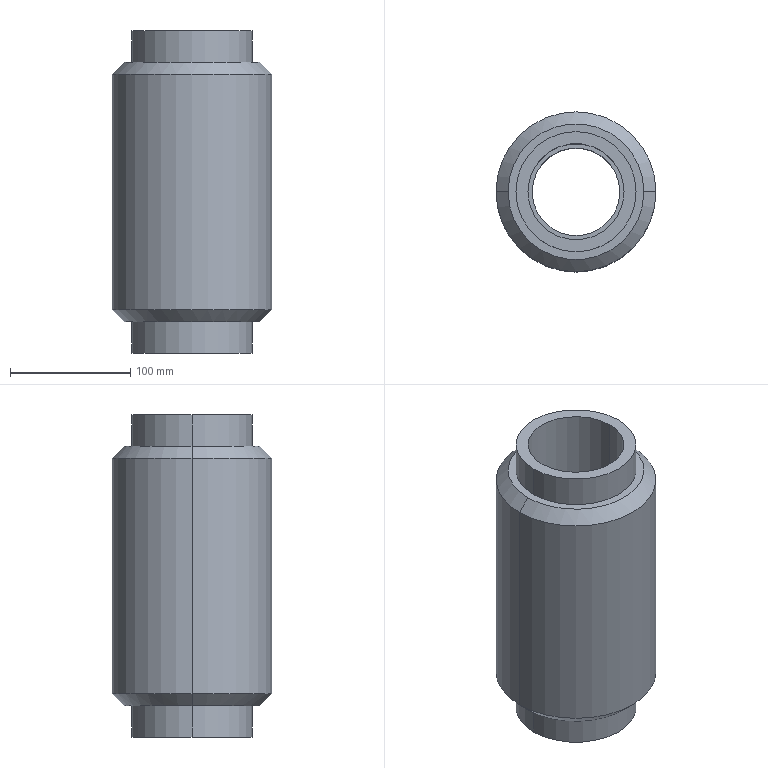Part | SolidWorks | features ICE 5, Chamfer 2, Extrusion 1 | 1 solid | 22 faces | box 133 x 133 x 268 mm | volume 2114999 mm3 | cylinder 12 | plane 6 | cone 4 | commonest cylinder face diameters 80 x4 100 x4 73 x2 133 x2
STEP:
#1=CARTESIAN_POINT('',(-56.5,0.,26.));
#2=VERTEX_POINT('',#1);
#3=CARTESIAN_POINT('',(56.5,0.,26.));
#4=VERTEX_POINT('',#3);
#5=CARTESIAN_POINT('',(0.,0.,26.));
#6=DIRECTION('',(0.,0.,-1.));
#7=DIRECTION('',(1.,0.,0.));
#8=AXIS2_PLACEMENT_3D('',#5,#6,#7);
#9=CIRCLE('',#8,56.5);
#10=EDGE_CURVE('',#2,#4,#9,.T.);
#11=ORIENTED_EDGE('',*,*,#10,.F.);
#12=CARTESIAN_POINT('',(-66.5,0.,36.));
#13=VERTEX_POINT('',#12);
#14=CARTESIAN_POINT('',(-66.5,0.,36.));
#15=DIRECTION('',(-0.7071,0.,0.7071));
#16=VECTOR('',#15,1000.);
#17=LINE('',#14,#16);
#18=EDGE_CURVE('',#2,#13,#17,.T.);
#19=ORIENTED_EDGE('',*,*,#18,.T.);
#20=CARTESIAN_POINT('',(66.5,0.,36.));
#21=VERTEX_POINT('',#20);
#22=CARTESIAN_POINT('',(0.,0.,36.));
#23=DIRECTION('',(0.,0.,1.));
#24=DIRECTION('',(1.,0.,0.));
#25=AXIS2_PLACEMENT_3D('',#22,#23,#24);
#26=CIRCLE('',#25,66.5);
#27=EDGE_CURVE('',#21,#13,#26,.T.);
#28=ORIENTED_EDGE('',*,*,#27,.F.);
#29=CARTESIAN_POINT('',(66.5,0.,36.));
#30=DIRECTION('',(0.7071,0.,0.7071));
#31=VECTOR('',#30,1000.);
#32=LINE('',#29,#31);
#33=EDGE_CURVE('',#4,#21,#32,.T.);
#34=ORIENTED_EDGE('',*,*,#33,.F.);
#35=EDGE_LOOP('',(#11,#19,#28,#34));
#36=FACE_OUTER_BOUND('',#35,.T.);
#37=CARTESIAN_POINT('',(0.,0.,36.));
#38=DIRECTION('',(0.,0.,1.));
#39=DIRECTION('',(1.,0.,0.));
#40=AXIS2_PLACEMENT_3D('',#37,#38,#39);
#41=CONICAL_SURFACE('',#40,66.5,0.7854);
#42=ADVANCED_FACE('',(#36),#41,.T.);
#43=CARTESIAN_POINT('',(56.5,0.,242.));
#44=VERTEX_POINT('',#43);
#45=CARTESIAN_POINT('',(-56.5,0.,242.));
#46=VERTEX_POINT('',#45);
#47=CARTESIAN_POINT('',(0.,0.,242.));
#48=DIRECTION('',(0.,0.,1.));
#49=DIRECTION('',(1.,0.,0.));
#50=AXIS2_PLACEMENT_3D('',#47,#48,#49);
#51=CIRCLE('',#50,56.5);
#52=EDGE_CURVE('',#44,#46,#51,.T.);
#53=ORIENTED_EDGE('',*,*,#52,.F.);
#54=CARTESIAN_POINT('',(66.5,0.,232.));
#55=VERTEX_POINT('',#54);
#56=CARTESIAN_POINT('',(56.5,0.,242.));
#57=DIRECTION('',(0.7071,0.,-0.7071));
#58=VECTOR('',#57,1000.);
#59=LINE('',#56,#58);
#60=EDGE_CURVE('',#44,#55,#59,.T.);
#61=ORIENTED_EDGE('',*,*,#60,.T.);
#62=CARTESIAN_POINT('',(-66.5,0.,232.));
#63=VERTEX_POINT('',#62);
#64=CARTESIAN_POINT('',(0.,0.,232.));
#65=DIRECTION('',(0.,0.,-1.));
#66=DIRECTION('',(1.,0.,0.));
#67=AXIS2_PLACEMENT_3D('',#64,#65,#66);
#68=CIRCLE('',#67,66.5);
#69=EDGE_CURVE('',#63,#55,#68,.T.);
#70=ORIENTED_EDGE('',*,*,#69,.F.);
#71=CARTESIAN_POINT('',(-56.5,0.,242.));
#72=DIRECTION('',(-0.7071,0.,-0.7071));
#73=VECTOR('',#72,1000.);
#74=LINE('',#71,#73);
#75=EDGE_CURVE('',#46,#63,#74,.T.);
#76=ORIENTED_EDGE('',*,*,#75,.F.);
#77=EDGE_LOOP('',(#53,#61,#70,#76));
#78=FACE_OUTER_BOUND('',#77,.T.);
#79=CARTESIAN_POINT('',(0.,0.,242.));
#80=DIRECTION('',(0.,0.,-1.));
#81=DIRECTION('',(-1.,0.,0.));
#82=AXIS2_PLACEMENT_3D('',#79,#80,#81);
#83=CONICAL_SURFACE('',#82,56.5,0.7854);
#84=ADVANCED_FACE('',(#78),#83,.T.);
#85=CARTESIAN_POINT('',(-36.5,0.,189.));
#86=VERTEX_POINT('',#85);
#87=CARTESIAN_POINT('',(36.5,0.,189.));
#88=VERTEX_POINT('',#87);
#89=CARTESIAN_POINT('',(0.,0.,189.));
#90=DIRECTION('',(0.,0.,1.));
#91=DIRECTION('',(1.,0.,0.));
#92=AXIS2_PLACEMENT_3D('',#89,#90,#91);
#93=CIRCLE('',#92,36.5);
#94=EDGE_CURVE('',#86,#88,#93,.T.);
#95=ORIENTED_EDGE('',*,*,#94,.T.);
#96=CARTESIAN_POINT('',(36.5,0.,79.));
#97=VERTEX_POINT('',#96);
#98=CARTESIAN_POINT('',(36.5,0.,268.));
#99=DIRECTION('',(0.,0.,-1.));
#100=VECTOR('',#99,1000.);
#101=LINE('',#98,#100);
#102=EDGE_CURVE('',#88,#97,#101,.T.);
#103=ORIENTED_EDGE('',*,*,#102,.T.);
#104=CARTESIAN_POINT('',(-36.5,0.,79.));
#105=VERTEX_POINT('',#104);
#106=CARTESIAN_POINT('',(0.,0.,79.));
#107=DIRECTION('',(0.,0.,-1.));
#108=DIRECTION('',(-1.,0.,0.));
#109=AXIS2_PLACEMENT_3D('',#106,#107,#108);
#110=CIRCLE('',#109,36.5);
#111=EDGE_CURVE('',#97,#105,#110,.T.);
#112=ORIENTED_EDGE('',*,*,#111,.T.);
#113=CARTESIAN_POINT('',(-36.5,0.,268.));
#114=DIRECTION('',(0.,0.,-1.));
#115=VECTOR('',#114,1000.);
#116=LINE('',#113,#115);
#117=EDGE_CURVE('',#86,#105,#116,.T.);
#118=ORIENTED_EDGE('',*,*,#117,.F.);
#119=EDGE_LOOP('',(#95,#103,#112,#118));
#120=FACE_OUTER_BOUND('',#119,.T.);
#121=CARTESIAN_POINT('',(0.,0.,268.));
#122=DIRECTION('',(0.,0.,-1.));
#123=DIRECTION('',(-1.,0.,0.));
#124=AXIS2_PLACEMENT_3D('',#121,#122,#123);
#125=CYLINDRICAL_SURFACE('',#124,36.5);
#126=ADVANCED_FACE('',(#120),#125,.F.);
#127=CARTESIAN_POINT('',(40.,0.,79.));
#128=VERTEX_POINT('',#127);
#129=CARTESIAN_POINT('',(-40.,0.,79.));
#130=VERTEX_POINT('',#129);
#131=CARTESIAN_POINT('',(0.,0.,79.));
#132=DIRECTION('',(0.,0.,-1.));
#133=DIRECTION('',(-1.,0.,0.));
#134=AXIS2_PLACEMENT_3D('',#131,#132,#133);
#135=CIRCLE('',#134,40.);
#136=EDGE_CURVE('',#128,#130,#135,.T.);
#137=ORIENTED_EDGE('',*,*,#136,.F.);
#138=CARTESIAN_POINT('',(40.,0.,0.));
#139=VERTEX_POINT('',#138);
#140=CARTESIAN_POINT('',(40.,0.,79.));
#141=DIRECTION('',(0.,0.,-1.));
#142=VECTOR('',#141,1000.);
#143=LINE('',#140,#142);
#144=EDGE_CURVE('',#128,#139,#143,.T.);
#145=ORIENTED_EDGE('',*,*,#144,.T.);
#146=CARTESIAN_POINT('',(-40.,0.,0.));
#147=VERTEX_POINT('',#146);
#148=CARTESIAN_POINT('',(0.,0.,0.));
#149=DIRECTION('',(0.,0.,-1.));
#150=DIRECTION('',(-1.,0.,0.));
#151=AXIS2_PLACEMENT_3D('',#148,#149,#150);
#152=CIRCLE('',#151,40.);
#153=EDGE_CURVE('',#139,#147,#152,.T.);
#154=ORIENTED_EDGE('',*,*,#153,.T.);
#155=CARTESIAN_POINT('',(-40.,0.,79.));
#156=DIRECTION('',(0.,0.,-1.));
#157=VECTOR('',#156,1000.);
#158=LINE('',#155,#157);
#159=EDGE_CURVE('',#130,#147,#158,.T.);
#160=ORIENTED_EDGE('',*,*,#159,.F.);
#161=EDGE_LOOP('',(#137,#145,#154,#160));
#162=FACE_OUTER_BOUND('',#161,.T.);
#163=CARTESIAN_POINT('',(0.,0.,79.));
#164=DIRECTION('',(0.,0.,-1.));
#165=DIRECTION('',(-1.,0.,0.));
#166=AXIS2_PLACEMENT_3D('',#163,#164,#165);
#167=CYLINDRICAL_SURFACE('',#166,40.);
#168=ADVANCED_FACE('',(#162),#167,.F.);
#169=CARTESIAN_POINT('',(-40.,0.,189.));
#170=VERTEX_POINT('',#169);
#171=CARTESIAN_POINT('',(40.,0.,189.));
#172=VERTEX_POINT('',#171);
#173=CARTESIAN_POINT('',(0.,0.,189.));
#174=DIRECTION('',(0.,0.,1.));
#175=DIRECTION('',(1.,0.,0.));
#176=AXIS2_PLACEMENT_3D('',#173,#174,#175);
#177=CIRCLE('',#176,40.);
#178=EDGE_CURVE('',#170,#172,#177,.T.);
#179=ORIENTED_EDGE('',*,*,#178,.F.);
#180=CARTESIAN_POINT('',(-40.,0.,268.));
#181=VERTEX_POINT('',#180);
#182=CARTESIAN_POINT('',(-40.,0.,189.));
#183=DIRECTION('',(0.,0.,1.));
#184=VECTOR('',#183,1000.);
#185=LINE('',#182,#184);
#186=EDGE_CURVE('',#170,#181,#185,.T.);
#187=ORIENTED_EDGE('',*,*,#186,.T.);
#188=CARTESIAN_POINT('',(40.,0.,268.));
#189=VERTEX_POINT('',#188);
#190=CARTESIAN_POINT('',(0.,0.,268.));
#191=DIRECTION('',(0.,0.,1.));
#192=DIRECTION('',(1.,0.,0.));
#193=AXIS2_PLACEMENT_3D('',#190,#191,#192);
#194=CIRCLE('',#193,40.);
#195=EDGE_CURVE('',#181,#189,#194,.T.);
#196=ORIENTED_EDGE('',*,*,#195,.T.);
#197=CARTESIAN_POINT('',(40.,0.,189.));
#198=DIRECTION('',(0.,0.,1.));
#199=VECTOR('',#198,1000.);
#200=LINE('',#197,#199);
#201=EDGE_CURVE('',#172,#189,#200,.T.);
#202=ORIENTED_EDGE('',*,*,#201,.F.);
#203=EDGE_LOOP('',(#179,#187,#196,#202));
#204=FACE_OUTER_BOUND('',#203,.T.);
#205=CARTESIAN_POINT('',(0.,0.,189.));
#206=DIRECTION('',(0.,0.,1.));
#207=DIRECTION('',(1.,0.,0.));
#208=AXIS2_PLACEMENT_3D('',#205,#206,#207);
#209=CYLINDRICAL_SURFACE('',#208,40.);
#210=ADVANCED_FACE('',(#204),#209,.F.);
#211=CARTESIAN_POINT('',(50.,0.,268.));
#212=VERTEX_POINT('',#211);
#213=CARTESIAN_POINT('',(-50.,0.,268.));
#214=VERTEX_POINT('',#213);
#215=CARTESIAN_POINT('',(0.,0.,268.));
#216=DIRECTION('',(0.,0.,1.));
#217=DIRECTION('',(1.,0.,0.));
#218=AXIS2_PLACEMENT_3D('',#215,#216,#217);
#219=CIRCLE('',#218,50.);
#220=EDGE_CURVE('',#212,#214,#219,.T.);
#221=ORIENTED_EDGE('',*,*,#220,.F.);
#222=CARTESIAN_POINT('',(50.,0.,242.));
#223=VERTEX_POINT('',#222);
#224=CARTESIAN_POINT('',(50.,0.,268.));
#225=DIRECTION('',(0.,0.,-1.));
#226=VECTOR('',#225,1000.);
#227=LINE('',#224,#226);
#228=EDGE_CURVE('',#212,#223,#227,.T.);
#229=ORIENTED_EDGE('',*,*,#228,.T.);
#230=CARTESIAN_POINT('',(-50.,0.,242.));
#231=VERTEX_POINT('',#230);
#232=CARTESIAN_POINT('',(0.,0.,242.));
#233=DIRECTION('',(0.,0.,1.));
#234=DIRECTION('',(1.,0.,0.));
#235=AXIS2_PLACEMENT_3D('',#232,#233,#234);
#236=CIRCLE('',#235,50.);
#237=EDGE_CURVE('',#223,#231,#236,.T.);
#238=ORIENTED_EDGE('',*,*,#237,.T.);
#239=CARTESIAN_POINT('',(-50.,0.,268.));
#240=DIRECTION('',(0.,0.,-1.));
#241=VECTOR('',#240,1000.);
#242=LINE('',#239,#241);
#243=EDGE_CURVE('',#214,#231,#242,.T.);
#244=ORIENTED_EDGE('',*,*,#243,.F.);
#245=EDGE_LOOP('',(#221,#229,#238,#244));
#246=FACE_OUTER_BOUND('',#245,.T.);
#247=CARTESIAN_POINT('',(0.,0.,268.));
#248=DIRECTION('',(0.,0.,-1.));
#249=DIRECTION('',(-1.,0.,0.));
#250=AXIS2_PLACEMENT_3D('',#247,#248,#249);
#251=CYLINDRICAL_SURFACE('',#250,50.);
#252=ADVANCED_FACE('',(#246),#251,.T.);
#253=ORIENTED_EDGE('',*,*,#69,.T.);
#254=CARTESIAN_POINT('',(66.5,0.,242.));
#255=DIRECTION('',(0.,0.,-1.));
#256=VECTOR('',#255,1000.);
#257=LINE('',#254,#256);
#258=EDGE_CURVE('',#55,#21,#257,.T.);
#259=ORIENTED_EDGE('',*,*,#258,.T.);
#260=ORIENTED_EDGE('',*,*,#27,.T.);
#261=CARTESIAN_POINT('',(-66.5,0.,242.));
#262=DIRECTION('',(0.,0.,-1.));
#263=VECTOR('',#262,1000.);
#264=LINE('',#261,#263);
#265=EDGE_CURVE('',#63,#13,#264,.T.);
#266=ORIENTED_EDGE('',*,*,#265,.F.);
#267=EDGE_LOOP('',(#253,#259,#260,#266));
#268=FACE_OUTER_BOUND('',#267,.T.);
#269=CARTESIAN_POINT('',(0.,0.,242.));
#270=DIRECTION('',(0.,0.,-1.));
#271=DIRECTION('',(-1.,0.,0.));
#272=AXIS2_PLACEMENT_3D('',#269,#270,#271);
#273=CYLINDRICAL_SURFACE('',#272,66.5);
#274=ADVANCED_FACE('',(#268),#273,.T.);
#275=CARTESIAN_POINT('',(50.,0.,26.));
#276=VERTEX_POINT('',#275);
#277=CARTESIAN_POINT('',(-50.,0.,26.));
#278=VERTEX_POINT('',#277);
#279=CARTESIAN_POINT('',(0.,0.,26.));
#280=DIRECTION('',(0.,0.,1.));
#281=DIRECTION('',(1.,0.,0.));
#282=AXIS2_PLACEMENT_3D('',#279,#280,#281);
#283=CIRCLE('',#282,50.);
#284=EDGE_CURVE('',#276,#278,#283,.T.);
#285=ORIENTED_EDGE('',*,*,#284,.F.);
#286=CARTESIAN_POINT('',(50.,0.,0.));
#287=VERTEX_POINT('',#286);
#288=CARTESIAN_POINT('',(50.,0.,26.));
#289=DIRECTION('',(0.,0.,-1.));
#290=VECTOR('',#289,1000.);
#291=LINE('',#288,#290);
#292=EDGE_CURVE('',#276,#287,#291,.T.);
#293=ORIENTED_EDGE('',*,*,#292,.T.);
#294=CARTESIAN_POINT('',(-50.,0.,0.));
#295=VERTEX_POINT('',#294);
#296=CARTESIAN_POINT('',(0.,0.,0.));
#297=DIRECTION('',(0.,0.,1.));
#298=DIRECTION('',(1.,0.,0.));
#299=AXIS2_PLACEMENT_3D('',#296,#297,#298);
#300=CIRCLE('',#299,50.);
#301=EDGE_CURVE('',#287,#295,#300,.T.);
#302=ORIENTED_EDGE('',*,*,#301,.T.);
#303=CARTESIAN_POINT('',(-50.,0.,26.));
#304=DIRECTION('',(0.,0.,-1.));
#305=VECTOR('',#304,1000.);
#306=LINE('',#303,#305);
#307=EDGE_CURVE('',#278,#295,#306,.T.);
#308=ORIENTED_EDGE('',*,*,#307,.F.);
#309=EDGE_LOOP('',(#285,#293,#302,#308));
#310=FACE_OUTER_BOUND('',#309,.T.);
#311=CARTESIAN_POINT('',(0.,0.,26.));
#312=DIRECTION('',(0.,0.,-1.));
#313=DIRECTION('',(-1.,0.,0.));
#314=AXIS2_PLACEMENT_3D('',#311,#312,#313);
#315=CYLINDRICAL_SURFACE('',#314,50.);
#316=ADVANCED_FACE('',(#310),#315,.T.);
#317=CARTESIAN_POINT('',(0.,0.,242.));
#318=DIRECTION('',(0.,0.,1.));
#319=DIRECTION('',(1.,0.,0.));
#320=AXIS2_PLACEMENT_3D('',#317,#318,#319);
#321=CIRCLE('',#320,56.5);
#322=EDGE_CURVE('',#46,#44,#321,.T.);
#323=ORIENTED_EDGE('',*,*,#322,.T.);
#324=ORIENTED_EDGE('',*,*,#52,.T.);
#325=EDGE_LOOP('',(#323,#324));
#326=FACE_OUTER_BOUND('',#325,.T.);
#327=CARTESIAN_POINT('',(0.,0.,242.));
#328=DIRECTION('',(0.,0.,1.));
#329=DIRECTION('',(1.,0.,0.));
#330=AXIS2_PLACEMENT_3D('',#327,#328,#329);
#331=CIRCLE('',#330,50.);
#332=EDGE_CURVE('',#231,#223,#331,.T.);
#333=ORIENTED_EDGE('',*,*,#332,.F.);
#334=ORIENTED_EDGE('',*,*,#237,.F.);
#335=EDGE_LOOP('',(#333,#334));
#336=FACE_BOUND('',#335,.T.);
#337=CARTESIAN_POINT('',(0.,0.,242.));
#338=DIRECTION('',(0.,0.,1.));
#339=DIRECTION('',(1.,0.,0.));
#340=AXIS2_PLACEMENT_3D('',#337,#338,#339);
#341=PLANE('',#340);
#342=ADVANCED_FACE('',(#326,#336),#341,.T.);
#343=ORIENTED_EDGE('',*,*,#292,.F.);
#344=CARTESIAN_POINT('',(0.,0.,26.));
#345=DIRECTION('',(0.,0.,1.));
#346=DIRECTION('',(1.,0.,0.));
#347=AXIS2_PLACEMENT_3D('',#344,#345,#346);
#348=CIRCLE('',#347,50.);
#349=EDGE_CURVE('',#278,#276,#348,.T.);
#350=ORIENTED_EDGE('',*,*,#349,.F.);
#351=ORIENTED_EDGE('',*,*,#307,.T.);
#352=CARTESIAN_POINT('',(0.,0.,0.));
#353=DIRECTION('',(0.,0.,1.));
#354=DIRECTION('',(1.,0.,0.));
#355=AXIS2_PLACEMENT_3D('',#352,#353,#354);
#356=CIRCLE('',#355,50.);
#357=EDGE_CURVE('',#295,#287,#356,.T.);
#358=ORIENTED_EDGE('',*,*,#357,.T.);
#359=EDGE_LOOP('',(#343,#350,#351,#358));
#360=FACE_OUTER_BOUND('',#359,.T.);
#361=CARTESIAN_POINT('',(0.,0.,26.));
#362=DIRECTION('',(0.,0.,-1.));
#363=DIRECTION('',(-1.,0.,0.));
#364=AXIS2_PLACEMENT_3D('',#361,#362,#363);
#365=CYLINDRICAL_SURFACE('',#364,50.);
#366=ADVANCED_FACE('',(#360),#365,.T.);
#367=CARTESIAN_POINT('',(0.,0.,0.));
#368=DIRECTION('',(0.,0.,-1.));
#369=DIRECTION('',(-1.,0.,0.));
#370=AXIS2_PLACEMENT_3D('',#367,#368,#369);
#371=CIRCLE('',#370,40.);
#372=EDGE_CURVE('',#147,#139,#371,.T.);
#373=ORIENTED_EDGE('',*,*,#372,.F.);
#374=ORIENTED_EDGE('',*,*,#153,.F.);
#375=EDGE_LOOP('',(#373,#374));
#376=FACE_BOUND('',#375,.T.);
#377=ORIENTED_EDGE('',*,*,#357,.F.);
#378=ORIENTED_EDGE('',*,*,#301,.F.);
#379=EDGE_LOOP('',(#377,#378));
#380=FACE_OUTER_BOUND('',#379,.T.);
#381=CARTESIAN_POINT('',(0.,0.,0.));
#382=DIRECTION('',(0.,0.,1.));
#383=DIRECTION('',(1.,0.,0.));
#384=AXIS2_PLACEMENT_3D('',#381,#382,#383);
#385=PLANE('',#384);
#386=ADVANCED_FACE('',(#376,#380),#385,.F.);
#387=CARTESIAN_POINT('',(0.,0.,26.));
#388=DIRECTION('',(0.,0.,-1.));
#389=DIRECTION('',(1.,0.,0.));
#390=AXIS2_PLACEMENT_3D('',#387,#388,#389);
#391=CIRCLE('',#390,56.5);
#392=EDGE_CURVE('',#4,#2,#391,.T.);
#393=ORIENTED_EDGE('',*,*,#392,.T.);
#394=ORIENTED_EDGE('',*,*,#10,.T.);
#395=EDGE_LOOP('',(#393,#394));
#396=FACE_OUTER_BOUND('',#395,.T.);
#397=ORIENTED_EDGE('',*,*,#349,.T.);
#398=ORIENTED_EDGE('',*,*,#284,.T.);
#399=EDGE_LOOP('',(#397,#398));
#400=FACE_BOUND('',#399,.T.);
#401=CARTESIAN_POINT('',(0.,0.,26.));
#402=DIRECTION('',(0.,0.,1.));
#403=DIRECTION('',(1.,0.,0.));
#404=AXIS2_PLACEMENT_3D('',#401,#402,#403);
#405=PLANE('',#404);
#406=ADVANCED_FACE('',(#396,#400),#405,.F.);
#407=ORIENTED_EDGE('',*,*,#258,.F.);
#408=CARTESIAN_POINT('',(0.,0.,232.));
#409=DIRECTION('',(0.,0.,-1.));
#410=DIRECTION('',(1.,0.,0.));
#411=AXIS2_PLACEMENT_3D('',#408,#409,#410);
#412=CIRCLE('',#411,66.5);
#413=EDGE_CURVE('',#55,#63,#412,.T.);
#414=ORIENTED_EDGE('',*,*,#413,.T.);
#415=ORIENTED_EDGE('',*,*,#265,.T.);
#416=CARTESIAN_POINT('',(0.,0.,36.));
#417=DIRECTION('',(0.,0.,1.));
#418=DIRECTION('',(1.,0.,0.));
#419=AXIS2_PLACEMENT_3D('',#416,#417,#418);
#420=CIRCLE('',#419,66.5);
#421=EDGE_CURVE('',#13,#21,#420,.T.);
#422=ORIENTED_EDGE('',*,*,#421,.T.);
#423=EDGE_LOOP('',(#407,#414,#415,#422));
#424=FACE_OUTER_BOUND('',#423,.T.);
#425=CARTESIAN_POINT('',(0.,0.,242.));
#426=DIRECTION('',(0.,0.,-1.));
#427=DIRECTION('',(-1.,0.,0.));
#428=AXIS2_PLACEMENT_3D('',#425,#426,#427);
#429=CYLINDRICAL_SURFACE('',#428,66.5);
#430=ADVANCED_FACE('',(#424),#429,.T.);
#431=ORIENTED_EDGE('',*,*,#228,.F.);
#432=CARTESIAN_POINT('',(0.,0.,268.));
#433=DIRECTION('',(0.,0.,1.));
#434=DIRECTION('',(1.,0.,0.));
#435=AXIS2_PLACEMENT_3D('',#432,#433,#434);
#436=CIRCLE('',#435,50.);
#437=EDGE_CURVE('',#214,#212,#436,.T.);
#438=ORIENTED_EDGE('',*,*,#437,.F.);
#439=ORIENTED_EDGE('',*,*,#243,.T.);
#440=ORIENTED_EDGE('',*,*,#332,.T.);
#441=EDGE_LOOP('',(#431,#438,#439,#440));
#442=FACE_OUTER_BOUND('',#441,.T.);
#443=CARTESIAN_POINT('',(0.,0.,268.));
#444=DIRECTION('',(0.,0.,-1.));
#445=DIRECTION('',(-1.,0.,0.));
#446=AXIS2_PLACEMENT_3D('',#443,#444,#445);
#447=CYLINDRICAL_SURFACE('',#446,50.);
#448=ADVANCED_FACE('',(#442),#447,.T.);
#449=CARTESIAN_POINT('',(0.,0.,268.));
#450=DIRECTION('',(0.,0.,1.));
#451=DIRECTION('',(1.,0.,0.));
#452=AXIS2_PLACEMENT_3D('',#449,#450,#451);
#453=CIRCLE('',#452,40.);
#454=EDGE_CURVE('',#189,#181,#453,.T.);
#455=ORIENTED_EDGE('',*,*,#454,.F.);
#456=ORIENTED_EDGE('',*,*,#195,.F.);
#457=EDGE_LOOP('',(#455,#456));
#458=FACE_BOUND('',#457,.T.);
#459=ORIENTED_EDGE('',*,*,#437,.T.);
#460=ORIENTED_EDGE('',*,*,#220,.T.);
#461=EDGE_LOOP('',(#459,#460));
#462=FACE_OUTER_BOUND('',#461,.T.);
#463=CARTESIAN_POINT('',(0.,0.,268.));
#464=DIRECTION('',(0.,0.,1.));
#465=DIRECTION('',(1.,0.,0.));
#466=AXIS2_PLACEMENT_3D('',#463,#464,#465);
#467=PLANE('',#466);
#468=ADVANCED_FACE('',(#458,#462),#467,.T.);
#469=ORIENTED_EDGE('',*,*,#186,.F.);
#470=CARTESIAN_POINT('',(0.,0.,189.));
#471=DIRECTION('',(0.,0.,1.));
#472=DIRECTION('',(1.,0.,0.));
#473=AXIS2_PLACEMENT_3D('',#470,#471,#472);
#474=CIRCLE('',#473,40.);
#475=EDGE_CURVE('',#172,#170,#474,.T.);
#476=ORIENTED_EDGE('',*,*,#475,.F.);
#477=ORIENTED_EDGE('',*,*,#201,.T.);
#478=ORIENTED_EDGE('',*,*,#454,.T.);
#479=EDGE_LOOP('',(#469,#476,#477,#478));
#480=FACE_OUTER_BOUND('',#479,.T.);
#481=CARTESIAN_POINT('',(0.,0.,189.));
#482=DIRECTION('',(0.,0.,1.));
#483=DIRECTION('',(1.,0.,0.));
#484=AXIS2_PLACEMENT_3D('',#481,#482,#483);
#485=CYLINDRICAL_SURFACE('',#484,40.);
#486=ADVANCED_FACE('',(#480),#485,.F.);
#487=ORIENTED_EDGE('',*,*,#94,.F.);
#488=CARTESIAN_POINT('',(0.,0.,189.));
#489=DIRECTION('',(0.,0.,1.));
#490=DIRECTION('',(1.,0.,0.));
#491=AXIS2_PLACEMENT_3D('',#488,#489,#490);
#492=CIRCLE('',#491,36.5);
#493=EDGE_CURVE('',#88,#86,#492,.T.);
#494=ORIENTED_EDGE('',*,*,#493,.F.);
#495=EDGE_LOOP('',(#487,#494));
#496=FACE_BOUND('',#495,.T.);
#497=ORIENTED_EDGE('',*,*,#475,.T.);
#498=ORIENTED_EDGE('',*,*,#178,.T.);
#499=EDGE_LOOP('',(#497,#498));
#500=FACE_OUTER_BOUND('',#499,.T.);
#501=CARTESIAN_POINT('',(0.,0.,189.));
#502=DIRECTION('',(0.,0.,1.));
#503=DIRECTION('',(1.,0.,0.));
#504=AXIS2_PLACEMENT_3D('',#501,#502,#503);
#505=PLANE('',#504);
#506=ADVANCED_FACE('',(#496,#500),#505,.T.);
#507=ORIENTED_EDGE('',*,*,#144,.F.);
#508=CARTESIAN_POINT('',(0.,0.,79.));
#509=DIRECTION('',(0.,0.,-1.));
#510=DIRECTION('',(-1.,0.,0.));
#511=AXIS2_PLACEMENT_3D('',#508,#509,#510);
#512=CIRCLE('',#511,40.);
#513=EDGE_CURVE('',#130,#128,#512,.T.);
#514=ORIENTED_EDGE('',*,*,#513,.F.);
#515=ORIENTED_EDGE('',*,*,#159,.T.);
#516=ORIENTED_EDGE('',*,*,#372,.T.);
#517=EDGE_LOOP('',(#507,#514,#515,#516));
#518=FACE_OUTER_BOUND('',#517,.T.);
#519=CARTESIAN_POINT('',(0.,0.,79.));
#520=DIRECTION('',(0.,0.,-1.));
#521=DIRECTION('',(-1.,0.,0.));
#522=AXIS2_PLACEMENT_3D('',#519,#520,#521);
#523=CYLINDRICAL_SURFACE('',#522,40.);
#524=ADVANCED_FACE('',(#518),#523,.F.);
#525=CARTESIAN_POINT('',(0.,0.,79.));
#526=DIRECTION('',(0.,0.,-1.));
#527=DIRECTION('',(-1.,0.,0.));
#528=AXIS2_PLACEMENT_3D('',#525,#526,#527);
#529=CIRCLE('',#528,36.5);
#530=EDGE_CURVE('',#105,#97,#529,.T.);
#531=ORIENTED_EDGE('',*,*,#530,.F.);
#532=ORIENTED_EDGE('',*,*,#111,.F.);
#533=EDGE_LOOP('',(#531,#532));
#534=FACE_BOUND('',#533,.T.);
#535=ORIENTED_EDGE('',*,*,#513,.T.);
#536=ORIENTED_EDGE('',*,*,#136,.T.);
#537=EDGE_LOOP('',(#535,#536));
#538=FACE_OUTER_BOUND('',#537,.T.);
#539=CARTESIAN_POINT('',(0.,0.,79.));
#540=DIRECTION('',(0.,0.,-1.));
#541=DIRECTION('',(-1.,0.,0.));
#542=AXIS2_PLACEMENT_3D('',#539,#540,#541);
#543=PLANE('',#542);
#544=ADVANCED_FACE('',(#534,#538),#543,.T.);
#545=ORIENTED_EDGE('',*,*,#102,.F.);
#546=ORIENTED_EDGE('',*,*,#493,.T.);
#547=ORIENTED_EDGE('',*,*,#117,.T.);
#548=ORIENTED_EDGE('',*,*,#530,.T.);
#549=EDGE_LOOP('',(#545,#546,#547,#548));
#550=FACE_OUTER_BOUND('',#549,.T.);
#551=CARTESIAN_POINT('',(0.,0.,268.));
#552=DIRECTION('',(0.,0.,-1.));
#553=DIRECTION('',(-1.,0.,0.));
#554=AXIS2_PLACEMENT_3D('',#551,#552,#553);
#555=CYLINDRICAL_SURFACE('',#554,36.5);
#556=ADVANCED_FACE('',(#550),#555,.F.);
#557=ORIENTED_EDGE('',*,*,#60,.F.);
#558=ORIENTED_EDGE('',*,*,#322,.F.);
#559=ORIENTED_EDGE('',*,*,#75,.T.);
#560=ORIENTED_EDGE('',*,*,#413,.F.);
#561=EDGE_LOOP('',(#557,#558,#559,#560));
#562=FACE_OUTER_BOUND('',#561,.T.);
#563=CARTESIAN_POINT('',(0.,0.,242.));
#564=DIRECTION('',(0.,0.,-1.));
#565=DIRECTION('',(-1.,0.,0.));
#566=AXIS2_PLACEMENT_3D('',#563,#564,#565);
#567=CONICAL_SURFACE('',#566,56.5,0.7854);
#568=ADVANCED_FACE('',(#562),#567,.T.);
#569=ORIENTED_EDGE('',*,*,#18,.F.);
#570=ORIENTED_EDGE('',*,*,#392,.F.);
#571=ORIENTED_EDGE('',*,*,#33,.T.);
#572=ORIENTED_EDGE('',*,*,#421,.F.);
#573=EDGE_LOOP('',(#569,#570,#571,#572));
#574=FACE_OUTER_BOUND('',#573,.T.);
#575=CARTESIAN_POINT('',(0.,0.,36.));
#576=DIRECTION('',(0.,0.,1.));
#577=DIRECTION('',(1.,0.,0.));
#578=AXIS2_PLACEMENT_3D('',#575,#576,#577);
#579=CONICAL_SURFACE('',#578,66.5,0.7854);
#580=ADVANCED_FACE('',(#574),#579,.T.);
#581=CLOSED_SHELL('',(#42,#84,#126,#168,#210,#252,#274,#316,#342,#366,#386,#406,#430,#448,#468,#486,#506,#524,#544,#556,#568,#580));
#582=MANIFOLD_SOLID_BREP('',#581);
#583=CARTESIAN_POINT('',(0.,0.,0.));
#584=DIRECTION('',(0.,0.,1.));
#585=DIRECTION('',(1.,0.,0.));
#586=AXIS2_PLACEMENT_3D('',#583,#584,#585);
#587=(LENGTH_UNIT()NAMED_UNIT(*)SI_UNIT(.MILLI.,.METRE.));
#588=UNCERTAINTY_MEASURE_WITH_UNIT(LENGTH_MEASURE(0.00001),#587,'','');
#589=(NAMED_UNIT(*)PLANE_ANGLE_UNIT()SI_UNIT($,.RADIAN.));
#590=(NAMED_UNIT(*)SI_UNIT($,.STERADIAN.)SOLID_ANGLE_UNIT());
#591=(GEOMETRIC_REPRESENTATION_CONTEXT(3)GLOBAL_UNCERTAINTY_ASSIGNED_CONTEXT((#588))GLOBAL_UNIT_ASSIGNED_CONTEXT((#587,#589,#590))REPRESENTATION_CONTEXT('',''));
#592=ADVANCED_BREP_SHAPE_REPRESENTATION('',(#582,#586),#591);